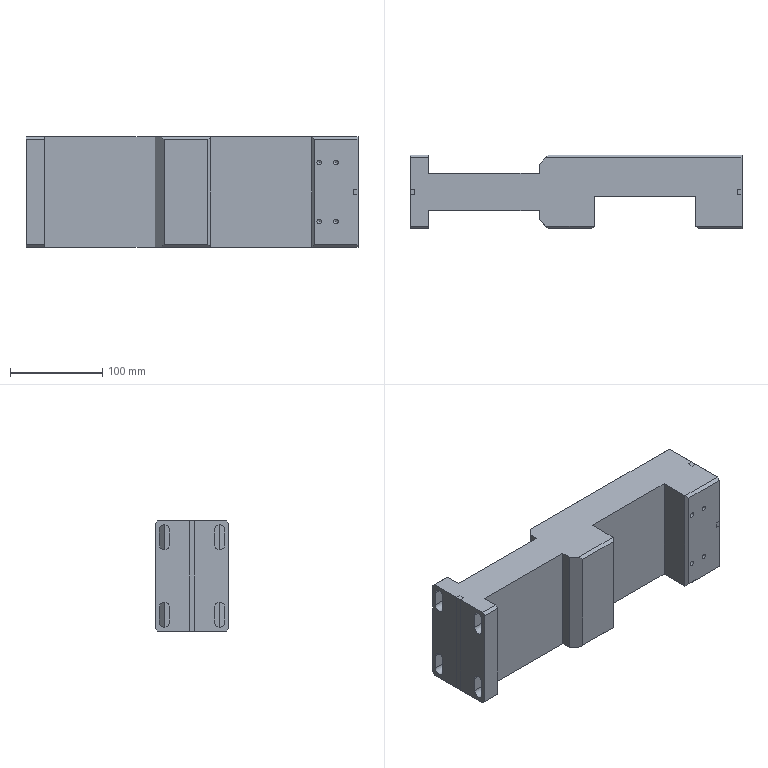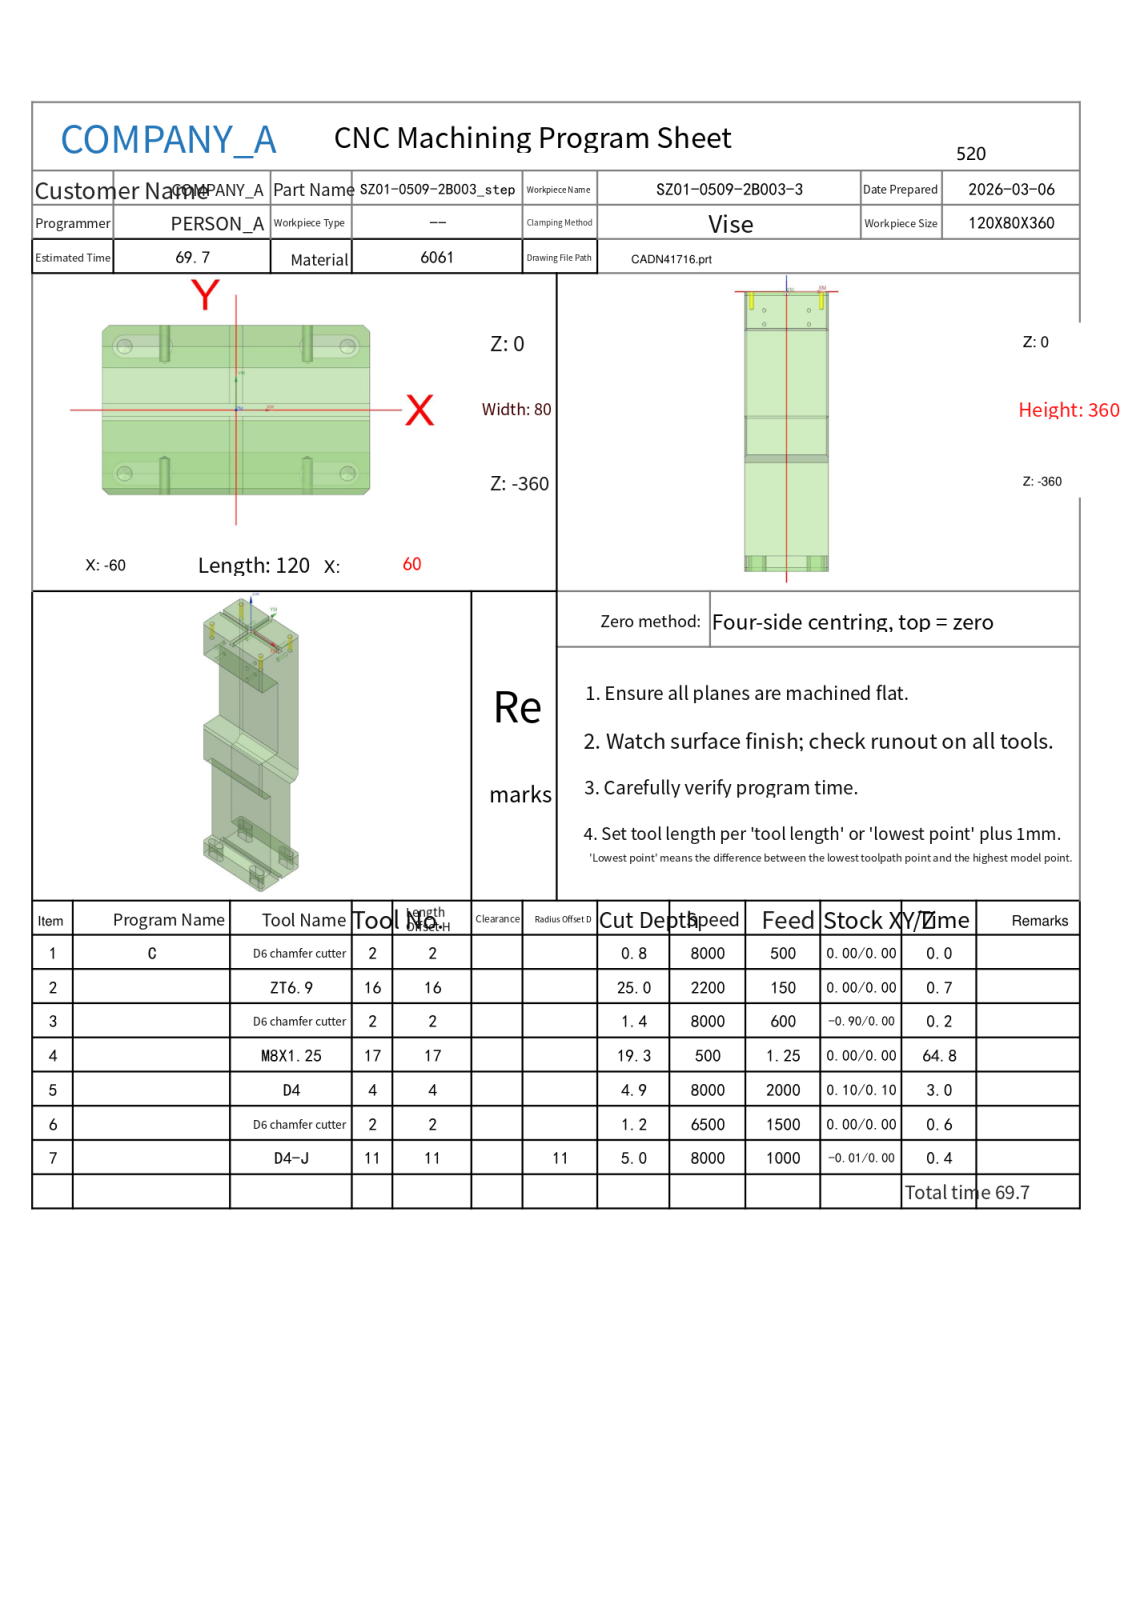NC program | NX | posted by the shop | part box 360 x 80 x 120 mm
Whole program:
%
O0001
(Machine time: 132.84 MIN)
(===Total Tool:5===)
(T2=D6 chamfer cutter   D=6.   R=0.   D-  H02 Z=-1.4  )
(T16=ZT6.9  D=6.9  DR_a=120 D-  H16 Z=-25.  )
(T17=M8X1.25 D=6.8  DR_a=180 D-  H17 Z=-19.25)
(T4=D4      D=4.   R=0.   D-  H04 Z=-4.9  )
(T11=D4-J   D=4.   R=0.   D11 H11 Z=-5.   )
G80 G90 G17 G49 G40
G91 G28 Z0
M01
N1 T02 M06
(D6 chamfer cutter  D=6. R=0. H=02 ce=0.00 di=0.00)
G00 G90 G54 X50. Y-30. M03 S8000
G43 H02 Z50.
M08
G98 G81 X50. Y-30. Z-.8 R1. F500.
Y30.
X-50.
Y-30.
G80
G00 Z50.
G91 G28 Z0.0
M05
M09
G91 G28 Z0.0
M01
N2 T16 M06
(ZT6.9 D=6.9 DR_a=120 H=16)
G00 G90 G54 X50. Y-30. M03 S2200
G43 H16 Z50.
M08
G98 G83 X50. Y-30. Z-25. R1. F150. Q2.
Y30.
X-50.
Y-30.
G80
G00 Z50.
G91 G28 Z0.0
M05
M09
G91 G28 Z0.0
M01
N3 T02 M06
(D6 chamfer cutter  D=6. R=0. H=02 ce=-0.90 di=0.00)
G00 G90 G54 X48.834 Y31.5 M03 S8000
G43 H02 Z50.
M08
Z-.9
G01 Z-1.4 F600.
X48.6
G03 X47.1 Y30. I0.0 J-1.5
X50. Y27.1 I2.9 J0.0
X52.9 Y30. I0.0 J2.9
X50. Y32.9 I-2.9 J0.0
X47.1 Y30. I0.0 J-2.9
X48.6 Y28.5 I1.5 J0.0
G01 X48.834
Z-.9
G00 Z50.
Y-28.5
Z-.9
G01 Z-1.4
X48.6
G03 X47.1 Y-30. I0.0 J-1.5
X50. Y-32.9 I2.9 J0.0
X52.9 Y-30. I0.0 J2.9
X50. Y-27.1 I-2.9 J0.0
X47.1 Y-30. I0.0 J-2.9
X48.6 Y-31.5 I1.5 J0.0
G01 X48.834
Z-.9
G00 Z50.
X-51.166 Y-28.5
Z-.9
G01 Z-1.4
X-51.4
G03 X-52.9 Y-30. I0.0 J-1.5
X-50. Y-32.9 I2.9 J0.0
X-47.1 Y-30. I0.0 J2.9
X-50. Y-27.1 I-2.9 J0.0
X-52.9 Y-30. I0.0 J-2.9
X-51.4 Y-31.5 I1.5 J0.0
G01 X-51.166
Z-.9
G00 Z50.
Y31.5
Z-.9
G01 Z-1.4
X-51.4
G03 X-52.9 Y30. I0.0 J-1.5
X-50. Y27.1 I2.9 J0.0
X-47.1 Y30. I0.0 J2.9
X-50. Y32.9 I-2.9 J0.0
X-52.9 Y30. I0.0 J-2.9
X-51.4 Y28.5 I1.5 J0.0
G01 X-51.166
Z-.9
G00 Z50.
G91 G28 Z0.0
M05
M09
G91 G28 Z0.0
M01
N4 T17 M06
(M8X1.25 D=6.8 DR_a=180 H=17)
G00 G90 G54 X50. Y-30. M03 S500
G43 H17 Z50.
M08
G95
G98 G84 X50. Y-30. Z-19.25 R1. F1.25 Q4.
Y30.
X-50.
Y-30.
G80
G94
G00 Z50.
G91 G28 Z0.0
M05
M09
G91 G28 Z0.0
M01
N5 T04 M06
(D4  D=4. R=0. H=04 ce=0.10 di=0.10)
G00 G90 G54 X65.1 Y0.0 M03 S8000
G43 H04 Z10.1
M08
Z1.15
G01 Z-.35 F2000.
X61.96
Y-.9
X.9
Y-41.96
X-.9
Y-.9
X-61.96
Y.9
X-.9
Y41.96
X.9
Y.9
X61.96
Y0.0
Y-.5
X65.1
Z1.15
G00 Y0.0
Z.8
G01 Z-.7
X61.96
Y-.9
X.9
Y-41.96
X-.9
Y-.9
X-61.96
Y.9
X-.9
Y41.96
X.9
Y.9
X61.96
Y0.0
Y-.5
X65.1
Z.8
G00 Y0.0
Z.45
G01 Z-1.05
X61.96
Y-.9
X.9
Y-41.96
X-.9
Y-.9
X-61.96
Y.9
X-.9
Y41.96
X.9
Y.9
X61.96
Y0.0
Y-.5
X65.1
Z.45
G00 Y0.0
Z.1
G01 Z-1.4
X61.96
Y-.9
X.9
Y-41.96
X-.9
Y-.9
X-61.96
Y.9
X-.9
Y41.96
X.9
Y.9
X61.96
Y0.0
Y-.5
X65.1
Z.1
G00 Y0.0
Z-.25
G01 Z-1.75
X61.96
Y-.9
X.9
Y-41.96
X-.9
Y-.9
X-61.96
Y.9
X-.9
Y41.96
X.9
Y.9
X61.96
Y0.0
Y-.5
X65.1
Z-.25
G00 Y0.0
Z-.6
G01 Z-2.1
X61.96
Y-.9
X.9
Y-41.96
X-.9
Y-.9
X-61.96
Y.9
X-.9
Y41.96
X.9
Y.9
X61.96
Y0.0
Y-.5
X65.1
Z-.6
G00 Y0.0
Z-.95
G01 Z-2.45
X61.96
Y-.9
X.9
Y-41.96
X-.9
Y-.9
X-61.96
Y.9
X-.9
Y41.96
X.9
Y.9
X61.96
Y0.0
Y-.5
X65.1
Z-.95
G00 Y0.0
Z-1.3
G01 Z-2.8
X61.96
Y-.9
X.9
Y-41.96
X-.9
Y-.9
X-61.96
Y.9
X-.9
Y41.96
X.9
Y.9
X61.96
Y0.0
Y-.5
X65.1
Z-1.3
G00 Y0.0
Z-1.65
G01 Z-3.15
X61.96
Y-.9
X.9
Y-41.96
X-.9
Y-.9
X-61.96
Y.9
X-.9
Y41.96
X.9
Y.9
X61.96
Y0.0
Y-.5
X65.1
Z-1.65
G00 Y0.0
Z-2.
G01 Z-3.5
X61.96
Y-.9
X.9
Y-41.96
X-.9
Y-.9
X-61.96
Y.9
X-.9
Y41.96
X.9
Y.9
X61.96
Y0.0
Y-.5
X65.1
Z-2.
G00 Y0.0
Z-2.35
G01 Z-3.85
X61.96
Y-.9
X.9
Y-41.96
X-.9
Y-.9
X-61.96
Y.9
X-.9
Y41.96
X.9
Y.9
X61.96
Y0.0
Y-.5
X65.1
Z-2.35
G00 Y0.0
Z-2.7
G01 Z-4.2
X61.96
Y-.9
X.9
Y-41.96
X-.9
Y-.9
X-61.96
Y.9
X-.9
Y41.96
X.9
Y.9
X61.96
Y0.0
Y-.5
X65.1
Z-2.7
G00 Y0.0
Z-3.05
G01 Z-4.55
X61.96
Y-.9
X.9
Y-41.96
X-.9
Y-.9
X-61.96
Y.9
X-.9
Y41.96
X.9
Y.9
X61.96
Y0.0
Y-.5
X65.1
Z-3.05
G00 Y0.0
Z-3.4
G01 Z-4.9
X61.96
Y-.9
X.9
Y-41.96
X-.9
Y-.9
X-61.96
Y.9
X-.9
Y41.96
X.9
Y.9
X61.96
Y0.0
Y-.5
X65.1
Z-3.4
G00 Z10.1
G91 G28 Z0.0
M05
M09
G91 G28 Z0.0
M01
N6 T02 M06
(D6 chamfer cutter  D=6. R=0. H=02 ce=0.00 di=0.00)
G00 G90 G54 X-31.886 Y-1.773 M03 S6500
G43 H02 Z50.
M08
Z.172
G01 Z-1.2 F1500.
G03 X-31.6 Y-1.973 I1.286 J1.532
G01 X-31.554 Y-2.003
X-31.5 Y-2.
X-3.
G02 X-2. Y-3. I0.0 J-1.
G01 Y-40.
G02 X-3. Y-41. I-1. J0.0
G01 X-57.
X-57.259 Y-40.966
X-57.5 Y-40.866
X-57.707 Y-40.707
X-60.707 Y-37.707
X-60.866 Y-37.5
X-60.966 Y-37.259
X-61. Y-37.
Y-3.
G02 X-60. Y-2. I1. J0.0
G01 X-31.5
X-31.446 Y-2.003
X-31.4 Y-1.973
G03 X-31.114 Y-1.773 I-1. J1.732
G01 Z.172
G00 Z10.
X-52.208 Y-29.596
Z.252
G01 Z-1.2
G03 X-52.382 Y-29.898 I1.638 J-1.147
G01 X-52.408 Y-29.946
X-52.4 Y-30.
G03 X-50. Y-32.4 I2.4 J0.0
X-47.6 Y-30. I0.0 J2.4
X-50. Y-27.6 I-2.4 J0.0
X-52.4 Y-30. I0.0 J-2.4
G01 X-52.408 Y-30.054
X-52.382 Y-30.102
G03 X-52.208 Y-30.404 I1.813 J.845
G01 Z.252
G00 Z10.
X-31.114 Y1.773
Z.172
G01 Z-1.2
G03 X-31.4 Y1.973 I-1.286 J-1.532
G01 X-31.446 Y2.003
X-31.5 Y2.
X-60.
G02 X-61. Y3. I0.0 J1.
G01 Y37.
X-60.966 Y37.259
X-60.866 Y37.5
X-60.707 Y37.707
X-57.707 Y40.707
X-57.5 Y40.866
X-57.259 Y40.966
X-57. Y41.
X-3.
G02 X-2. Y40. I0.0 J-1.
G01 Y3.
G02 X-3. Y2. I-1. J0.0
G01 X-31.5
X-31.554 Y2.003
X-31.6 Y1.973
G03 X-31.886 Y1.773 I1. J-1.732
G01 Z.172
G00 Z10.
X-52.208 Y30.404
Z.252
G01 Z-1.2
G03 X-52.382 Y30.102 I1.638 J-1.147
G01 X-52.408 Y30.054
X-52.4 Y30.
G03 X-50. Y27.6 I2.4 J0.0
X-47.6 Y30. I0.0 J2.4
X-50. Y32.4 I-2.4 J0.0
X-52.4 Y30. I0.0 J-2.4
G01 X-52.408 Y29.946
X-52.382 Y29.898
G03 X-52.208 Y29.596 I1.813 J.845
G01 Z.252
G00 Z10.
X31.886 Y1.773
Z.172
G01 Z-1.2
G03 X31.6 Y1.973 I-1.286 J-1.532
G01 X31.554 Y2.003
X31.5 Y2.
X3.
G02 X2. Y3. I0.0 J1.
G01 Y40.
G02 X3. Y41. I1. J0.0
G01 X57.
X57.259 Y40.966
X57.5 Y40.866
X57.707 Y40.707
X60.707 Y37.707
X60.866 Y37.5
X60.966 Y37.259
X61. Y37.
Y3.
G02 X60. Y2. I-1. J0.0
G01 X31.5
X31.446 Y2.003
X31.4 Y1.973
G03 X31.114 Y1.773 I1. J-1.732
G01 Z.172
G00 Z10.
X47.792 Y30.404
Z.252
G01 Z-1.2
G03 X47.618 Y30.102 I1.638 J-1.147
G01 X47.592 Y30.054
X47.6 Y30.
G03 X50. Y27.6 I2.4 J0.0
X52.4 Y30. I0.0 J2.4
X50. Y32.4 I-2.4 J0.0
X47.6 Y30. I0.0 J-2.4
G01 X47.592 Y29.946
X47.618 Y29.898
G03 X47.792 Y29.596 I1.813 J.845
G01 Z.252
G00 Z10.
X31.114 Y-1.773
Z.172
G01 Z-1.2
G03 X31.4 Y-1.973 I1.286 J1.532
G01 X31.446 Y-2.003
X31.5 Y-2.
X60.
G02 X61. Y-3. I0.0 J-1.
G01 Y-37.
X60.966 Y-37.259
X60.866 Y-37.5
X60.707 Y-37.707
X57.707 Y-40.707
X57.5 Y-40.866
X57.259 Y-40.966
X57. Y-41.
X3.
G02 X2. Y-40. I0.0 J1.
G01 Y-3.
G02 X3. Y-2. I1. J0.0
G01 X31.5
X31.554 Y-2.003
X31.6 Y-1.973
G03 X31.886 Y-1.773 I-1. J1.732
G01 Z.172
G00 Z10.
X47.792 Y-29.596
Z.252
G01 Z-1.2
G03 X47.618 Y-29.898 I1.638 J-1.147
G01 X47.592 Y-29.946
X47.6 Y-30.
G03 X50. Y-32.4 I2.4 J0.0
X52.4 Y-30. I0.0 J2.4
X50. Y-27.6 I-2.4 J0.0
X47.6 Y-30. I0.0 J-2.4
G01 X47.592 Y-30.054
X47.618 Y-30.102
G03 X47.792 Y-30.404 I1.813 J.845
G01 Z.252
G00 Z50.
G91 G28 Z0.0
M05
M09
G91 G28 Z0.0
M01
N7 T11 M06
(D4-J  D=4. R=0. H=11 ce=-0.01 di=0.00)
G00 G90 G54 X-62.824 Y-.173 M03 S8000
G43 H11 Z10.001
M08
Z-4.
G01 Z-5. F1000.
G41 D11
X-62.785 Y-.369
G03 X-62. Y-1.015 I.785 J.154
G01 X-1.015
Y-42.
G03 X-.369 Y-42.785 I.8 J0.0
G01 G40 X-.173 Y-42.824
X.173
G41 D11
X.369 Y-42.785
G03 X1.015 Y-42. I-.154 J.785
G01 Y-1.015
X62.
G03 X62.785 Y-.369 I0.0 J.8
G01 G40 X62.824 Y-.173
Y.173
G41 D11
X62.785 Y.369
G03 X62. Y1.015 I-.785 J-.154
G01 X1.015
Y42.
G03 X.369 Y42.785 I-.8 J0.0
G01 G40 X.173 Y42.824
X-.173
G41 D11
X-.369 Y42.785
G03 X-1.015 Y42. I.154 J-.785
G01 Y1.015
X-62.
G03 X-62.785 Y.369 I0.0 J-.8
G01 G40 X-62.824 Y.173
Z-4.
G00 Z10.001
M05
M09
G91 G28 Z0.0
G91 G28 Y0.0
M30
%